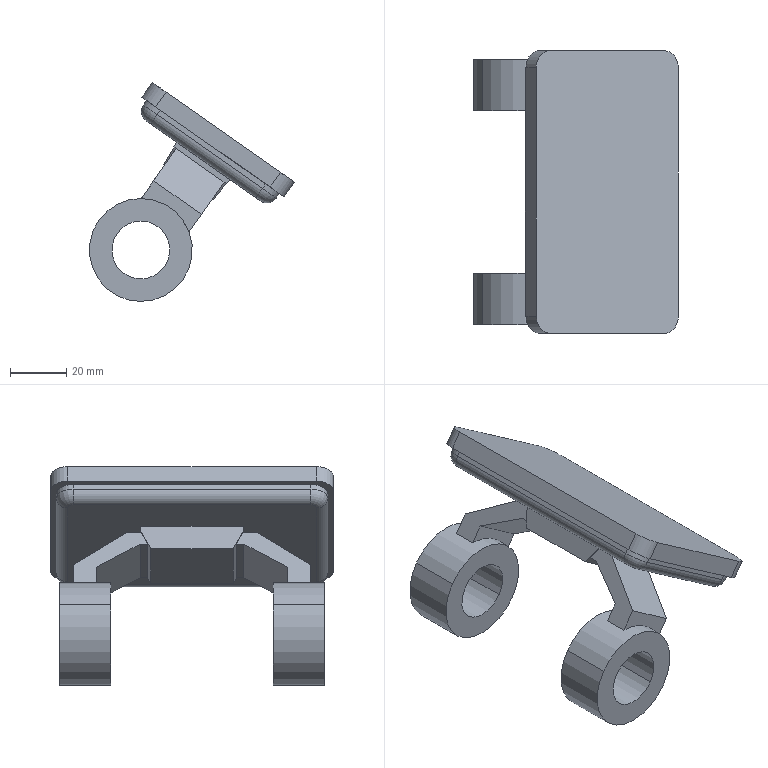Part | SolidWorks | features BaseBody 1 | 1 solid | 62 faces | box 73.029 x 100.7 x 78.014 mm | volume 113164 mm3 | plane 38 | cylinder 20 | torus 4 | commonest cylinder face diameters 12 x8 8 x4 20.6 x4 36.7 x4